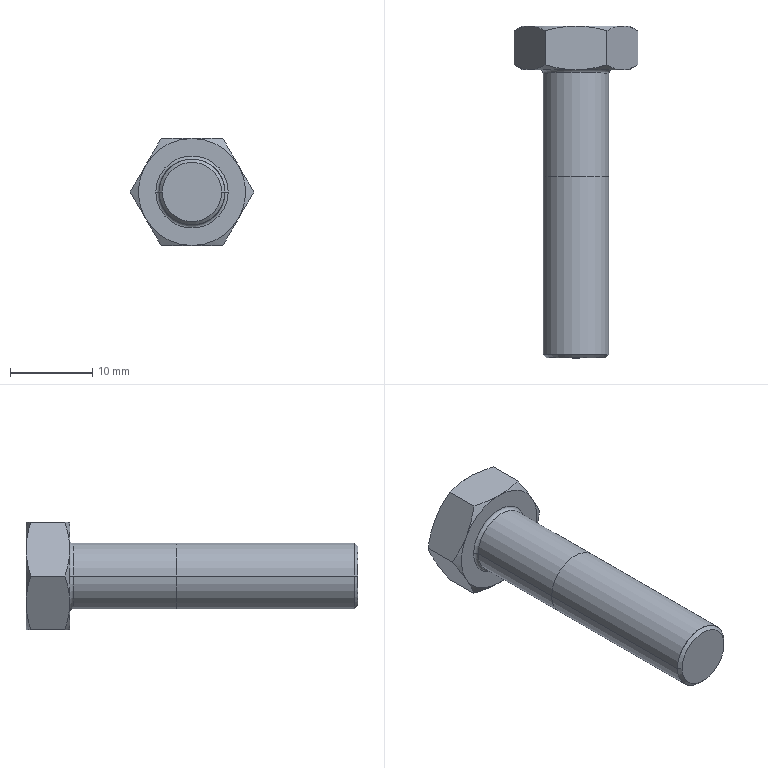Part | NX | features BREP 2 | 1 solid | 31 faces | box 15.011 x 40.3 x 13 mm | volume 2917 mm3 | cone 14 | plane 11 | cylinder 4 | torus 2 | commonest cylinder face diameters 6.647 x2 8 x2